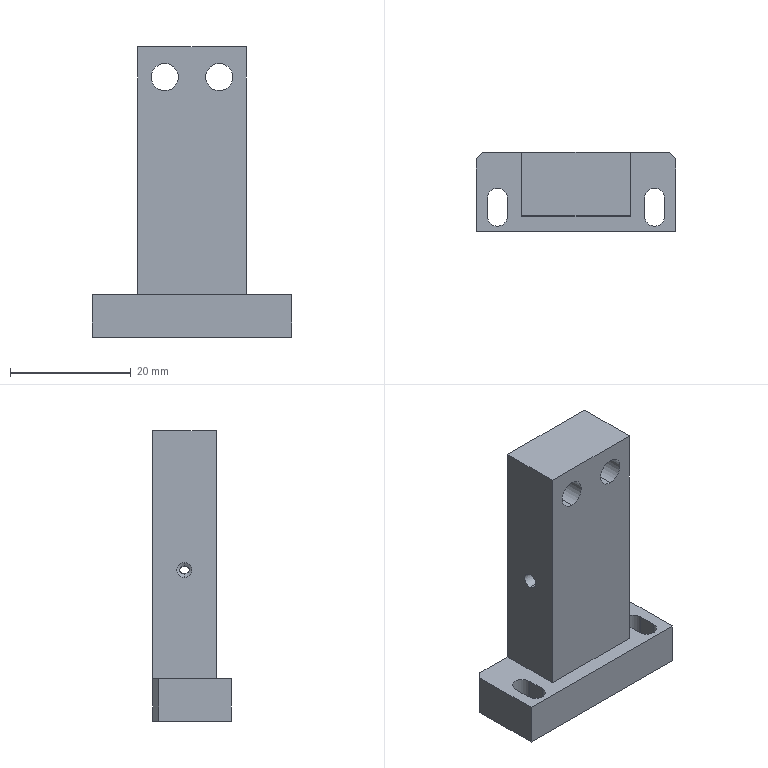Part | STEP file | 1 solid | 42 faces | box 33 x 13 x 48 mm | volume 9695 mm3 | cylinder 18 | plane 18 | cone 6 | commonest cylinder face diameters 2.5 x6 3.3 x4 4.5 x4 8 x4